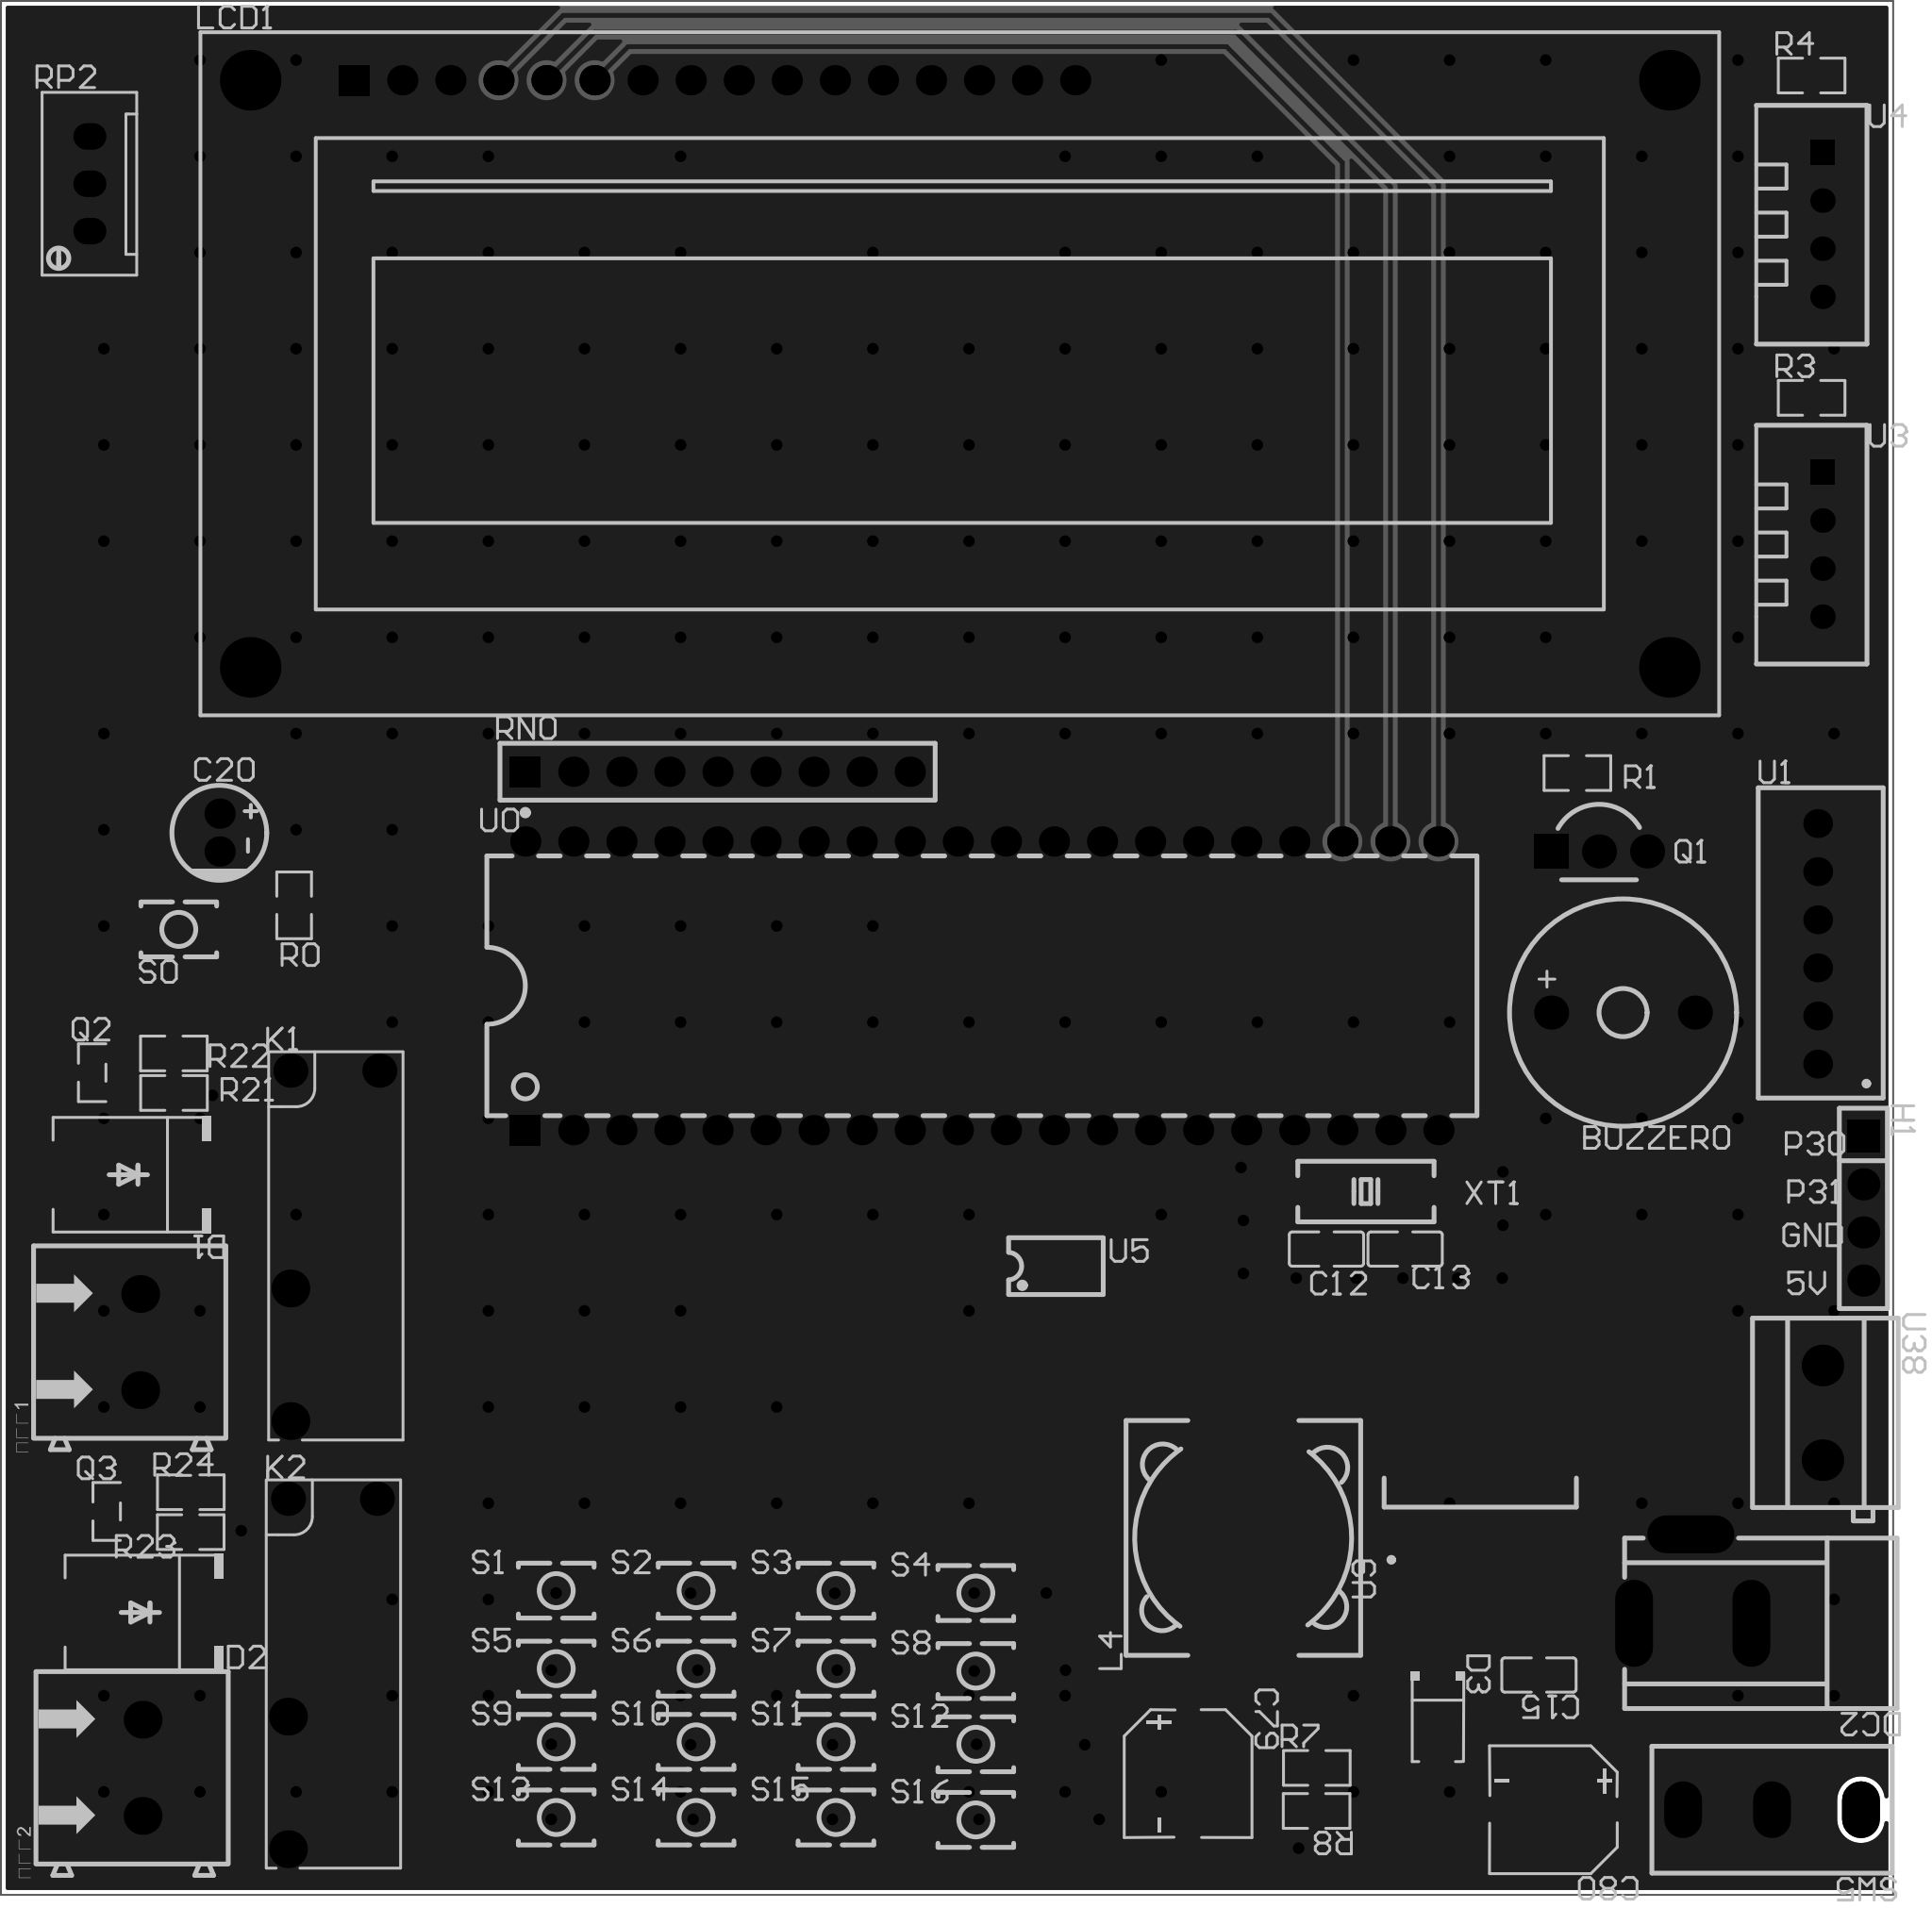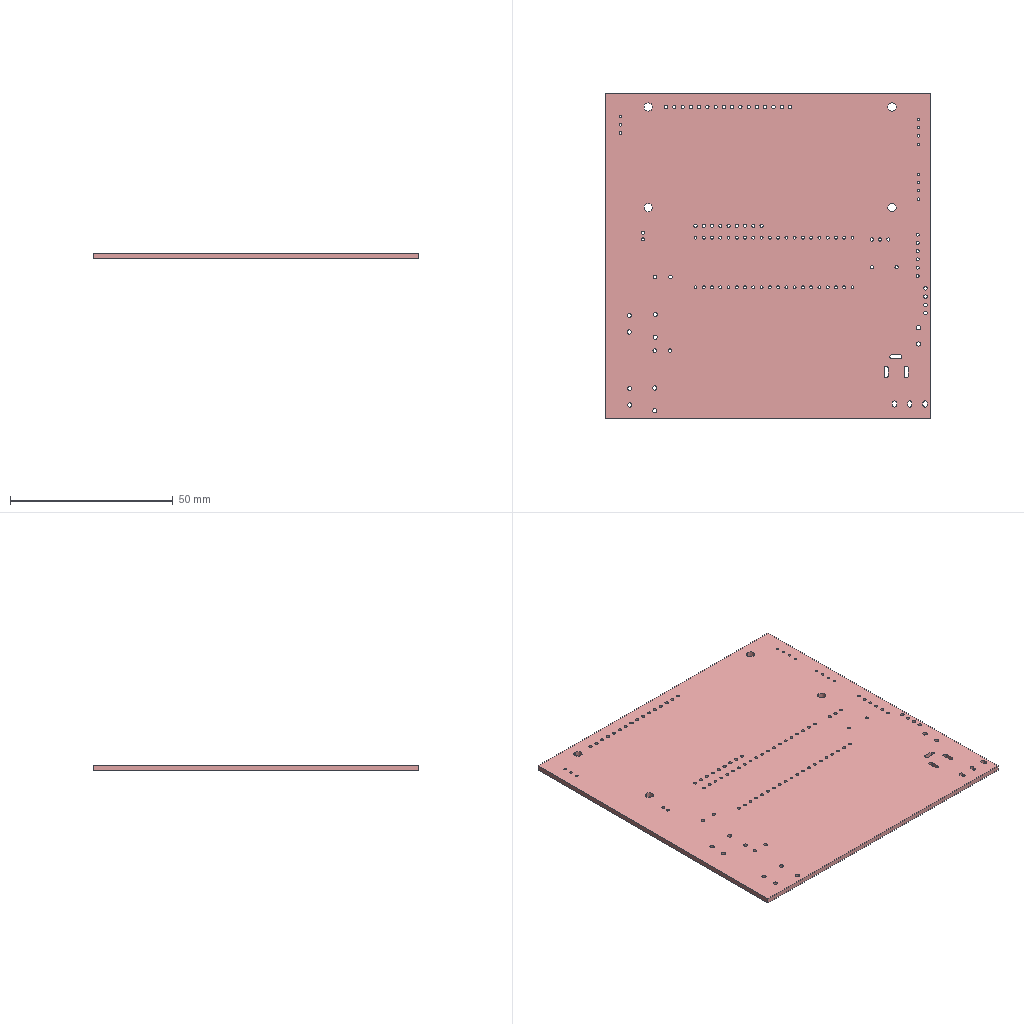Circuit board layout | Altium Designer | box 100 x 100 x 1.6 mm
Layer stack:
# Altium Designer layer stack of  (unit mm; dielectric type: 0 none, 1 core, 2 prepreg, 3 surface material)
index,name,kind,layer,copper_thickness_mm,dielectric_type,dielectric_thickness_mm,dielectric_material,dielectric_constant
0,Top Paste Mask Layer,other,,,,,,
1,Top Silkscreen Layer,other,,,,,,
2,Top Solder Mask Layer,dielectric,,,3,0.01,,3.3
3,Top Layer,copper,Top Layer,0.035,,,,
4,Dielectric1,dielectric,,,3,1.51,FR4,4.5
5,Bottom Layer,copper,Bottom Layer,0.035,,,,
6,Bottom Solder Mask Layer,dielectric,,,3,0.01,,3.3
7,Bottom Silkscreen Layer,other,,,,,,
8,Bottom Paste Mask Layer,other,,,,,,
# drill layer pairs: low layer,high layer
drill_pair,Top Layer,Bottom Layer
Part placement:
Designator,Comment,Layer,Footprint,Center-X(mm),Center-Y(mm),Rotation
BUZZER0,2.4kHz,TopLayer,BUZ-TH_BD12.0-P7.60-D0.6-FD,174.117,137.087,0
C15,100nF,TopLayer,C0805,169.672,102.108,180
C79,100uF,TopLayer,CAP-SMD_BD6.3-L6.6-W6.6-LS7.4-FD,151.13,96.901,270
C80,100uF,TopLayer,CAP-SMD_BD6.3-L6.6-W6.6-LS7.4-FD,170.434,94.996,180
D1,,TopLayer,SMC_L6.9-W5.9-LS7.9-RD,95.123,128.524,180
D2,,TopLayer,SMC_L6.9-W5.9-LS7.9-RD,95.758,105.41,180
D3,SS510,TopLayer,SMA_L4.3-W2.6-LS5.0-RD,164.338,99.695,270
DC2,DC005,TopLayer,DC-IN-TH_DC005,177.8,107.188,180
K1,,TopLayer,RELAY-TH_G5NB-1A-E-DCXX,106.04,124.767,270
K2,,TopLayer,RELAY-TH_G5NB-1A-E-DCXX,105.913,102.161,270
L4,47uH,TopLayer,IND-SMD_L12.3-W12.3,154.051,109.347,90
LCD1,LCD 1602,TopLayer,LCD1602,139.065,170.815,0
Q1,SS8550DTA,TopLayer,TO-92-3_L4.8-W3.7-P2.54-L,172.847,145.596,0
Q2,S8050(0.5A),TopLayer,SOT-23-3_L2.9-W1.3-P1.90-LS2.4-BR,93.213,133.911,0
Q3,S8050(0.5A),TopLayer,SOT-23-3_L2.9-W1.3-P1.90-LS2.4-BR,93.98,110.744,0
R1,5.1K,TopLayer,R0805,171.704,149.733,0
R3,10K,TopLayer,R0805,184.083,169.545,0
R4,10K,TopLayer,R0805,184.083,186.563,0
R7,3.3K,TopLayer,R0805,157.933,97.202,0
R8,10K,TopLayer,R0805,157.922,94.929,180
R21,4.7K,TopLayer,R0805,97.536,132.842,0
R22,4.7K,TopLayer,R0805,97.531,134.927,180
R23,4.7K,TopLayer,R0805,98.42,109.654,0
R24,4.7K,TopLayer,R0805,98.425,111.76,180
RN0,10kΩ,TopLayer,RES-ARRAY-TH_9P-P2.54-D1.0,126.263,149.803,0
RP2,10K,TopLayer,RES-ADJ-TH_3296W-1-203,93.091,180.848,270
S1,SW2,TopLayer,SW-SMD_L3.9-W2.9-LS5.0,117.737,106.564,0
S2,SW2,TopLayer,SW-SMD_L3.9-W2.9-LS5.0,125.128,106.564,0
S3,SW2,TopLayer,SW-SMD_L3.9-W2.9-LS5.0,132.52,106.564,0
S4,SW2,TopLayer,SW-SMD_L3.9-W2.9-LS5.0,139.911,106.437,0
S5,SW2,TopLayer,SW-SMD_L3.9-W2.9-LS5.0,117.737,102.444,0
S6,SW2,TopLayer,SW-SMD_L3.9-W2.9-LS5.0,125.128,102.444,0
S7,SW2,TopLayer,SW-SMD_L3.9-W2.9-LS5.0,132.52,102.444,0
S8,SW2,TopLayer,SW-SMD_L3.9-W2.9-LS5.0,139.911,102.317,0
S9,SW2,TopLayer,SW-SMD_L3.9-W2.9-LS5.0,117.737,98.578,0
S10,SW2,TopLayer,SW-SMD_L3.9-W2.9-LS5.0,125.128,98.578,0
S11,SW2,TopLayer,SW-SMD_L3.9-W2.9-LS5.0,132.52,98.578,0
S12,SW2,TopLayer,SW-SMD_L3.9-W2.9-LS5.0,139.911,98.451,0
S13,SW2,TopLayer,SW-SMD_L3.9-W2.9-LS5.0,117.737,94.585,0
S14,SW2,TopLayer,SW-SMD_L3.9-W2.9-LS5.0,125.128,94.585,0
S15,SW2,TopLayer,SW-SMD_L3.9-W2.9-LS5.0,132.52,94.585,0
S16,SW2,TopLayer,SW-SMD_L3.9-W2.9-LS5.0,139.911,94.458,0
SW5,SS-12D10L5,TopLayer,SW-TH_SS-12D10L5,181.991,94.996,180
U0,STC89C52RC-40I-PDIP40,TopLayer,DIP-40_L52.0-W13.7-P2.54-LS15.2-BL,140.233,138.5,0
U1,HM-10,TopLayer,HM-10.288,184.404,140.716,180
U3,DHT11,TopLayer,SENSOR-TH_DHT11,184.658,161.798,270
U4,DHT11,TopLayer,SENSOR-TH_DHT11,184.658,178.689,270
U5,M24C64-RMN6TP,TopLayer,SOIC-8_L5.0-W4.0-P1.27-LS6.0-BL,144.145,123.698,0
U9,XL4015E1,TopLayer,TO-263-5_L10.2-W8.9-P1.70-TL,166.57,112.941,90
U38,KF301-5.0-2P,TopLayer,CONN-TH_P5.00_KF301-5.0-2P,184.658,115.951,270
外接口1,,TopLayer,CONN-TH_2P-P5.00_WJ500V-5.08-2P,95.753,119.687,90
外接口2,,TopLayer,CONN-TH_2P-P5.00_WJ500V-5.08-2P,95.88,97.208,90
C12,30pf,TopLayer,C0805,158.441,124.6,180
C13,30pf,TopLayer,C0805,162.6,124.6,0
C20,CAP-E,TopLayer,CAP-TH_BD5.0-P2.00-D0.5-FD-A,99.949,146.59,270
R0,10K,TopLayer,R0805,103.886,142.748,90
S0,SW2,TopLayer,SW-SMD_L3.9-W2.9-LS5.0,97.79,141.478,180
XT1,XT,TopLayer,HC-49S_L7.2-W3.2,160.528,127.635,180
H1,,TopLayer,HDR-TH_4P-P2.54-V-F,186.817,126.746,270
Pad and via stacks:
# Altium Designer via and pad stacks of  (unit mm). Each distinct definition once, with the count of objects using it.
# via: kind,start_layer,end_layer,hole_mm,diameter_mm,mode(0 simple;1 top-mid-bottom;2 full stack),diameter_per_layer,count,example_net
# pad: kind,layer,hole_mm,hole_type(0 round;1 square;2 slot),plating,top_size,top_shape(1 round;2 rect;3 octagon;9 rounded rect),mid_size,bottom_size,mode,footprint,size_per_layer,count,example
pad,Multi-Layer,1,0,plated,1.8x1.8,1,1.8x1.8,1.8x1.8,0,BUZ-TH_BD12.0-P7.60-D0.6-FD,,2,BUZZER0.2
pad,Multi-Layer,1.2,2,plated,2x4.6,1,2x4.6,2x4.6,0,DC-IN-TH_DC005,,2,DC2.1
pad,Multi-Layer,1.2,2,plated,4.6x2,1,4.6x2,4.6x2,0,DC-IN-TH_DC005,,1,DC2.3
pad,Multi-Layer,1.1,0,plated,1.8x1.8,1,1.8x1.8,1.8x1.8,0,RELAY-TH_G5NB-1A-E-DCXX,,4,K1.4
pad,Multi-Layer,1.3,0,plated,2x2,1,2x2,2x2,0,RELAY-TH_G5NB-1A-E-DCXX,,4,K1.2
pad,Multi-Layer,1,0,plated,1.6x1.6,1,1.6x1.6,1.6x1.6,0,LCD1602,,15,LCD1.16
pad,Multi-Layer,1,0,plated,1.6x1.6,2,1.6x1.6,1.6x1.6,0,LCD1602,,1,LCD1.1
pad,Multi-Layer,2.5,2,plated,3.2x3.2,1,3.2x3.2,3.2x3.2,0,LCD1602,,4,LCD1.0
pad,Multi-Layer,1,0,plated,1.8x1.8,1,1.8x1.8,1.8x1.8,0,TO-92-3_L4.8-W3.7-P2.54-L,,2,Q1.3
pad,Multi-Layer,1,0,plated,1.8x1.8,2,1.8x1.8,1.8x1.8,0,TO-92-3_L4.8-W3.7-P2.54-L,,1,Q1.1
pad,Multi-Layer,1,0,plated,1.6x1.6,2,1.6x1.6,1.6x1.6,0,RES-ARRAY-TH_9P-P2.54-D1.0,,1,RN0.1
pad,Multi-Layer,1,0,plated,1.6x1.6,1,1.6x1.6,1.6x1.6,0,RES-ARRAY-TH_9P-P2.54-D1.0,,8,RN0.2
pad,Multi-Layer,0.8,0,plated,1.4x1.75,1,1.4x1.75,1.4x1.75,0,RES-ADJ-TH_3296W-1-203,,3,RP2.1
pad,Multi-Layer,1.3,2,plated,2x3,1,2x3,2x3,0,SW-TH_SS-12D10L5,,3,SW5.1
pad,Multi-Layer,0.889,0,plated,1.6x1.6,1,1.6x1.6,1.6x1.6,0,DIP-40_L52.0-W13.7-P2.54-LS15.2-BL,,39,U0.31
pad,Multi-Layer,0.889,0,plated,1.6x1.6,2,1.6x1.6,1.6x1.6,0,DIP-40_L52.0-W13.7-P2.54-LS15.2-BL,,1,U0.1
pad,Multi-Layer,0.9144,0,plated,1.524x1.524,1,1.524x1.524,1.524x1.524,0,HM-10.288,,6,U1.1
pad,Multi-Layer,0.7112,0,plated,1.295x1.295,2,1.295x1.295,1.295x1.295,0,SENSOR-TH_DHT11,,2,U3.1
pad,Multi-Layer,0.7112,0,plated,1.295x1.295,1,1.295x1.295,1.295x1.295,0,SENSOR-TH_DHT11,,6,U3.2
pad,Multi-Layer,1.4,0,plated,2.2x2.2,1,2.2x2.2,2.2x2.2,0,CONN-TH_P5.00_KF301-5.0-2P,,2,U38.1
pad,Multi-Layer,1.3,0,plated,2x2,1,2x2,2x2,0,CONN-TH_2P-P5.00_WJ500V-5.08-2P,,4,\u5916\u63A5\u53E31.2
pad,Multi-Layer,0.9,0,plated,1.6x1.6,1,1.6x1.6,1.6x1.6,0,CAP-TH_BD5.0-P2.00-D0.5-FD-A,,2,C20.2
pad,Multi-Layer,1.1,0,plated,1.7x1.7,2,1.7x1.7,1.7x1.7,0,HDR-TH_4P-P2.54-V-F,,1,H1.1
pad,Multi-Layer,1.1,0,plated,1.7x1.7,1,1.7x1.7,1.7x1.7,0,HDR-TH_4P-P2.54-V-F,,3,H1.2
pad,Top Layer,0,0,plated,1.41x1.35,2,1.41x1.35,1.41x1.35,0,C0805,,6,C15.2
pad,Top Layer,0,0,plated,3.5x1.2,2,3.5x1.2,3.5x1.2,0,CAP-SMD_BD6.3-L6.6-W6.6-LS7.4-FD,,4,C79.1
pad,Top Layer,0,0,plated,2.7x3.3,2,2.7x3.3,2.7x3.3,0,SMC_L6.9-W5.9-LS7.9-RD,,4,D1.2
pad,Top Layer,0,0,plated,2.046x1.62,2,2.046x1.62,2.046x1.62,0,SMA_L4.3-W2.6-LS5.0-RD,,2,D3.2
pad,Top Layer,0,0,plated,2.9x5.4,2,2.9x5.4,2.9x5.4,0,IND-SMD_L12.3-W12.3,,2,L4.1
pad,Top Layer,0,0,plated,1x0.65,2,1x0.65,1x0.65,0,SOT-23-3_L2.9-W1.3-P1.90-LS2.4-BR,,6,Q2.1
pad,Top Layer,0,0,plated,1.133x1.377,2,1.133x1.377,1.133x1.377,0,R0805,,20,R1.2
pad,Top Layer,0,0,plated,1.5x2,2,1.5x2,1.5x2,0,SW-SMD_L3.9-W2.9-LS5.0,,34,S1.1
pad,Top Layer,0,0,plated,0.5684x1.95,1,0.5684x1.95,0.5684x1.95,0,SOIC-8_L5.0-W4.0-P1.27-LS6.0-BL,,8,U5.1
pad,Top Layer,0,0,plated,3.2x1.15,2,3.2x1.15,3.2x1.15,0,TO-263-5_L10.2-W8.9-P1.70-TL,,5,U9.5
pad,Top Layer,0,0,plated,3.852x3.852,1,3.852x3.852,3.852x3.852,0,TO-263-5_L10.2-W8.9-P1.70-TL,,1,U9.6
pad,Top Layer,0,0,plated,4.1x1.2,2,4.1x1.2,4.1x1.2,0,HC-49S_L7.2-W3.2,,2,XT1.1
via,Top Layer,Bottom Layer,0.3048,0.61,0,,246,P14
Copper pours:
name,layer,net,type(0 solid;1 hatched;2 none)
Top Layer-GND,Top Layer,GND,0
Bottom Layer-GND,Bottom Layer,GND,0